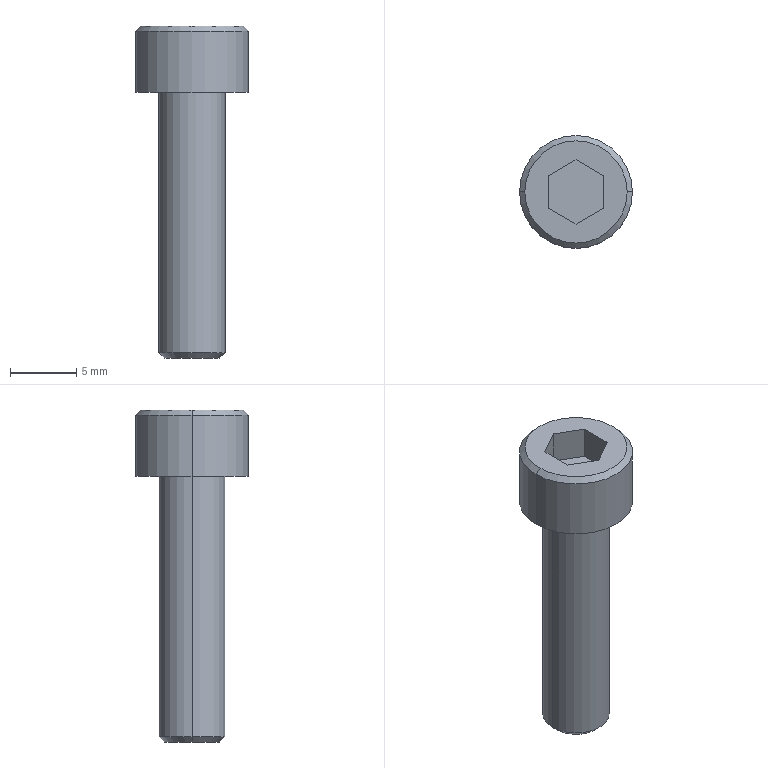Part | Creo | 1 solid | 18 faces | box 8.5 x 8.5 x 25 mm | volume 634.974 mm3 | plane 10 | cone 4 | cylinder 4 | commonest cylinder face diameters 5 x2 8.5 x2
STEP:
#1=CARTESIAN_POINT('',(95.85,150.15,32.599));
#2=VERTEX_POINT('',#1);
#3=CARTESIAN_POINT('',(88.15,150.15,32.599));
#4=VERTEX_POINT('',#3);
#5=CARTESIAN_POINT('',(92.,150.15,32.599));
#6=DIRECTION('',(0.,0.,1.));
#7=DIRECTION('',(1.,0.,0.));
#8=AXIS2_PLACEMENT_3D('',#5,#6,#7);
#9=CIRCLE('',#8,3.85);
#10=EDGE_CURVE('',#2,#4,#9,.T.);
#11=ORIENTED_EDGE('',*,*,#10,.F.);
#12=CARTESIAN_POINT('',(92.,150.15,32.599));
#13=DIRECTION('',(0.,0.,1.));
#14=DIRECTION('',(-1.,0.,0.));
#15=AXIS2_PLACEMENT_3D('',#12,#13,#14);
#16=CIRCLE('',#15,3.85);
#17=EDGE_CURVE('',#4,#2,#16,.T.);
#18=ORIENTED_EDGE('',*,*,#17,.F.);
#19=EDGE_LOOP('',(#11,#18));
#20=FACE_OUTER_BOUND('',#19,.F.);
#21=CARTESIAN_POINT('',(89.9,148.937,32.599));
#22=VERTEX_POINT('',#21);
#23=CARTESIAN_POINT('',(89.9,151.362,32.599));
#24=VERTEX_POINT('',#23);
#25=CARTESIAN_POINT('',(89.9,148.937,32.599));
#26=DIRECTION('',(0.,1.,0.));
#27=VECTOR('',#26,2.425);
#28=LINE('',#25,#27);
#29=EDGE_CURVE('',#22,#24,#28,.T.);
#30=ORIENTED_EDGE('',*,*,#29,.F.);
#31=CARTESIAN_POINT('',(92.,147.725,32.599));
#32=VERTEX_POINT('',#31);
#33=CARTESIAN_POINT('',(92.,147.725,32.599));
#34=DIRECTION('',(-0.866,0.5,0.));
#35=VECTOR('',#34,2.425);
#36=LINE('',#33,#35);
#37=EDGE_CURVE('',#32,#22,#36,.T.);
#38=ORIENTED_EDGE('',*,*,#37,.F.);
#39=CARTESIAN_POINT('',(94.1,148.937,32.599));
#40=VERTEX_POINT('',#39);
#41=CARTESIAN_POINT('',(94.1,148.937,32.599));
#42=DIRECTION('',(-0.866,-0.5,0.));
#43=VECTOR('',#42,2.425);
#44=LINE('',#41,#43);
#45=EDGE_CURVE('',#40,#32,#44,.T.);
#46=ORIENTED_EDGE('',*,*,#45,.F.);
#47=CARTESIAN_POINT('',(94.1,151.362,32.599));
#48=VERTEX_POINT('',#47);
#49=CARTESIAN_POINT('',(94.1,151.362,32.599));
#50=DIRECTION('',(0.,-1.,0.));
#51=VECTOR('',#50,2.425);
#52=LINE('',#49,#51);
#53=EDGE_CURVE('',#48,#40,#52,.T.);
#54=ORIENTED_EDGE('',*,*,#53,.F.);
#55=CARTESIAN_POINT('',(92.,152.575,32.599));
#56=VERTEX_POINT('',#55);
#57=CARTESIAN_POINT('',(92.,152.575,32.599));
#58=DIRECTION('',(0.866,-0.5,0.));
#59=VECTOR('',#58,2.425);
#60=LINE('',#57,#59);
#61=EDGE_CURVE('',#56,#48,#60,.T.);
#62=ORIENTED_EDGE('',*,*,#61,.F.);
#63=CARTESIAN_POINT('',(89.9,151.362,32.599));
#64=DIRECTION('',(0.866,0.5,0.));
#65=VECTOR('',#64,2.425);
#66=LINE('',#63,#65);
#67=EDGE_CURVE('',#24,#56,#66,.T.);
#68=ORIENTED_EDGE('',*,*,#67,.F.);
#69=EDGE_LOOP('',(#30,#38,#46,#54,#62,#68));
#70=FACE_BOUND('',#69,.F.);
#71=CARTESIAN_POINT('',(92.,150.15,32.599));
#72=DIRECTION('',(0.,0.,1.));
#73=DIRECTION('',(1.,0.,0.));
#74=AXIS2_PLACEMENT_3D('',#71,#72,#73);
#75=PLANE('',#74);
#76=ADVANCED_FACE('',(#20,#70),#75,.T.);
#77=ORIENTED_EDGE('',*,*,#10,.T.);
#78=CARTESIAN_POINT('',(87.75,150.15,32.199));
#79=VERTEX_POINT('',#78);
#80=CARTESIAN_POINT('',(88.15,150.15,32.599));
#81=DIRECTION('',(-0.7071,0.,-0.7071));
#82=VECTOR('',#81,0.5657);
#83=LINE('',#80,#82);
#84=EDGE_CURVE('',#4,#79,#83,.T.);
#85=ORIENTED_EDGE('',*,*,#84,.T.);
#86=CARTESIAN_POINT('',(96.25,150.15,32.199));
#87=VERTEX_POINT('',#86);
#88=CARTESIAN_POINT('',(92.,150.15,32.199));
#89=DIRECTION('',(0.,0.,1.));
#90=DIRECTION('',(1.,0.,0.));
#91=AXIS2_PLACEMENT_3D('',#88,#89,#90);
#92=CIRCLE('',#91,4.25);
#93=EDGE_CURVE('',#87,#79,#92,.T.);
#94=ORIENTED_EDGE('',*,*,#93,.F.);
#95=CARTESIAN_POINT('',(95.85,150.15,32.599));
#96=DIRECTION('',(0.7071,0.,-0.7071));
#97=VECTOR('',#96,0.5657);
#98=LINE('',#95,#97);
#99=EDGE_CURVE('',#2,#87,#98,.T.);
#100=ORIENTED_EDGE('',*,*,#99,.F.);
#101=EDGE_LOOP('',(#77,#85,#94,#100));
#102=FACE_OUTER_BOUND('',#101,.F.);
#103=CARTESIAN_POINT('',(92.,150.15,32.399));
#104=DIRECTION('',(0.,0.,-1.));
#105=DIRECTION('',(-1.,0.,0.));
#106=AXIS2_PLACEMENT_3D('',#103,#104,#105);
#107=CONICAL_SURFACE('',#106,4.05,45.);
#108=ADVANCED_FACE('',(#102),#107,.T.);
#109=ORIENTED_EDGE('',*,*,#17,.T.);
#110=ORIENTED_EDGE('',*,*,#99,.T.);
#111=CARTESIAN_POINT('',(92.,150.15,32.199));
#112=DIRECTION('',(0.,0.,1.));
#113=DIRECTION('',(-1.,0.,0.));
#114=AXIS2_PLACEMENT_3D('',#111,#112,#113);
#115=CIRCLE('',#114,4.25);
#116=EDGE_CURVE('',#79,#87,#115,.T.);
#117=ORIENTED_EDGE('',*,*,#116,.F.);
#118=ORIENTED_EDGE('',*,*,#84,.F.);
#119=EDGE_LOOP('',(#109,#110,#117,#118));
#120=FACE_OUTER_BOUND('',#119,.F.);
#121=CARTESIAN_POINT('',(92.,150.15,32.399));
#122=DIRECTION('',(0.,0.,-1.));
#123=DIRECTION('',(-1.,0.,0.));
#124=AXIS2_PLACEMENT_3D('',#121,#122,#123);
#125=CONICAL_SURFACE('',#124,4.05,45.);
#126=ADVANCED_FACE('',(#120),#125,.T.);
#127=ORIENTED_EDGE('',*,*,#116,.T.);
#128=CARTESIAN_POINT('',(96.25,150.15,27.599));
#129=VERTEX_POINT('',#128);
#130=CARTESIAN_POINT('',(96.25,150.15,27.599));
#131=DIRECTION('',(0.,0.,1.));
#132=VECTOR('',#131,4.6);
#133=LINE('',#130,#132);
#134=EDGE_CURVE('',#129,#87,#133,.T.);
#135=ORIENTED_EDGE('',*,*,#134,.F.);
#136=CARTESIAN_POINT('',(87.75,150.15,27.599));
#137=VERTEX_POINT('',#136);
#138=CARTESIAN_POINT('',(92.,150.15,27.599));
#139=DIRECTION('',(0.,0.,-1.));
#140=DIRECTION('',(1.,0.,0.));
#141=AXIS2_PLACEMENT_3D('',#138,#139,#140);
#142=CIRCLE('',#141,4.25);
#143=EDGE_CURVE('',#129,#137,#142,.T.);
#144=ORIENTED_EDGE('',*,*,#143,.T.);
#145=CARTESIAN_POINT('',(87.75,150.15,27.599));
#146=DIRECTION('',(0.,0.,1.));
#147=VECTOR('',#146,4.6);
#148=LINE('',#145,#147);
#149=EDGE_CURVE('',#137,#79,#148,.T.);
#150=ORIENTED_EDGE('',*,*,#149,.T.);
#151=EDGE_LOOP('',(#127,#135,#144,#150));
#152=FACE_OUTER_BOUND('',#151,.F.);
#153=CARTESIAN_POINT('',(92.,150.15,27.599));
#154=DIRECTION('',(0.,0.,1.));
#155=DIRECTION('',(1.,0.,0.));
#156=AXIS2_PLACEMENT_3D('',#153,#154,#155);
#157=CYLINDRICAL_SURFACE('',#156,4.25);
#158=ADVANCED_FACE('',(#152),#157,.T.);
#159=ORIENTED_EDGE('',*,*,#93,.T.);
#160=ORIENTED_EDGE('',*,*,#149,.F.);
#161=CARTESIAN_POINT('',(92.,150.15,27.599));
#162=DIRECTION('',(0.,0.,-1.));
#163=DIRECTION('',(-1.,0.,0.));
#164=AXIS2_PLACEMENT_3D('',#161,#162,#163);
#165=CIRCLE('',#164,4.25);
#166=EDGE_CURVE('',#137,#129,#165,.T.);
#167=ORIENTED_EDGE('',*,*,#166,.T.);
#168=ORIENTED_EDGE('',*,*,#134,.T.);
#169=EDGE_LOOP('',(#159,#160,#167,#168));
#170=FACE_OUTER_BOUND('',#169,.F.);
#171=CARTESIAN_POINT('',(92.,150.15,27.599));
#172=DIRECTION('',(0.,0.,1.));
#173=DIRECTION('',(1.,0.,0.));
#174=AXIS2_PLACEMENT_3D('',#171,#172,#173);
#175=CYLINDRICAL_SURFACE('',#174,4.25);
#176=ADVANCED_FACE('',(#170),#175,.T.);
#177=ORIENTED_EDGE('',*,*,#143,.F.);
#178=ORIENTED_EDGE('',*,*,#166,.F.);
#179=EDGE_LOOP('',(#177,#178));
#180=FACE_OUTER_BOUND('',#179,.F.);
#181=CARTESIAN_POINT('',(89.5,150.15,27.599));
#182=VERTEX_POINT('',#181);
#183=CARTESIAN_POINT('',(94.5,150.15,27.599));
#184=VERTEX_POINT('',#183);
#185=CARTESIAN_POINT('',(92.,150.15,27.599));
#186=DIRECTION('',(0.,0.,1.));
#187=DIRECTION('',(-1.,0.,0.));
#188=AXIS2_PLACEMENT_3D('',#185,#186,#187);
#189=CIRCLE('',#188,2.5);
#190=EDGE_CURVE('',#182,#184,#189,.T.);
#191=ORIENTED_EDGE('',*,*,#190,.F.);
#192=CARTESIAN_POINT('',(92.,150.15,27.599));
#193=DIRECTION('',(0.,0.,1.));
#194=DIRECTION('',(1.,0.,0.));
#195=AXIS2_PLACEMENT_3D('',#192,#193,#194);
#196=CIRCLE('',#195,2.5);
#197=EDGE_CURVE('',#184,#182,#196,.T.);
#198=ORIENTED_EDGE('',*,*,#197,.F.);
#199=EDGE_LOOP('',(#191,#198));
#200=FACE_BOUND('',#199,.F.);
#201=CARTESIAN_POINT('',(92.,150.15,27.599));
#202=DIRECTION('',(0.,0.,-1.));
#203=DIRECTION('',(-1.,0.,0.));
#204=AXIS2_PLACEMENT_3D('',#201,#202,#203);
#205=PLANE('',#204);
#206=ADVANCED_FACE('',(#180,#200),#205,.T.);
#207=CARTESIAN_POINT('',(94.5,150.15,7.999));
#208=VERTEX_POINT('',#207);
#209=CARTESIAN_POINT('',(89.5,150.15,7.999));
#210=VERTEX_POINT('',#209);
#211=CARTESIAN_POINT('',(92.,150.15,7.999));
#212=DIRECTION('',(0.,0.,-1.));
#213=DIRECTION('',(1.,0.,0.));
#214=AXIS2_PLACEMENT_3D('',#211,#212,#213);
#215=CIRCLE('',#214,2.5);
#216=EDGE_CURVE('',#208,#210,#215,.T.);
#217=ORIENTED_EDGE('',*,*,#216,.T.);
#218=CARTESIAN_POINT('',(89.5,150.15,27.599));
#219=DIRECTION('',(0.,0.,-1.));
#220=VECTOR('',#219,19.6);
#221=LINE('',#218,#220);
#222=EDGE_CURVE('',#182,#210,#221,.T.);
#223=ORIENTED_EDGE('',*,*,#222,.F.);
#224=ORIENTED_EDGE('',*,*,#190,.T.);
#225=CARTESIAN_POINT('',(94.5,150.15,27.599));
#226=DIRECTION('',(0.,0.,-1.));
#227=VECTOR('',#226,19.6);
#228=LINE('',#225,#227);
#229=EDGE_CURVE('',#184,#208,#228,.T.);
#230=ORIENTED_EDGE('',*,*,#229,.T.);
#231=EDGE_LOOP('',(#217,#223,#224,#230));
#232=FACE_OUTER_BOUND('',#231,.F.);
#233=CARTESIAN_POINT('',(92.,150.15,27.599));
#234=DIRECTION('',(0.,0.,-1.));
#235=DIRECTION('',(-1.,0.,0.));
#236=AXIS2_PLACEMENT_3D('',#233,#234,#235);
#237=CYLINDRICAL_SURFACE('',#236,2.5);
#238=ADVANCED_FACE('',(#232),#237,.T.);
#239=CARTESIAN_POINT('',(94.1,150.15,7.599));
#240=VERTEX_POINT('',#239);
#241=CARTESIAN_POINT('',(89.9,150.15,7.599));
#242=VERTEX_POINT('',#241);
#243=CARTESIAN_POINT('',(92.,150.15,7.599));
#244=DIRECTION('',(0.,0.,-1.));
#245=DIRECTION('',(1.,0.,0.));
#246=AXIS2_PLACEMENT_3D('',#243,#244,#245);
#247=CIRCLE('',#246,2.1);
#248=EDGE_CURVE('',#240,#242,#247,.T.);
#249=ORIENTED_EDGE('',*,*,#248,.T.);
#250=CARTESIAN_POINT('',(89.9,150.15,7.599));
#251=DIRECTION('',(-0.7071,0.,0.7071));
#252=VECTOR('',#251,0.5657);
#253=LINE('',#250,#252);
#254=EDGE_CURVE('',#242,#210,#253,.T.);
#255=ORIENTED_EDGE('',*,*,#254,.T.);
#256=ORIENTED_EDGE('',*,*,#216,.F.);
#257=CARTESIAN_POINT('',(94.1,150.15,7.599));
#258=DIRECTION('',(0.7071,0.,0.7071));
#259=VECTOR('',#258,0.5657);
#260=LINE('',#257,#259);
#261=EDGE_CURVE('',#240,#208,#260,.T.);
#262=ORIENTED_EDGE('',*,*,#261,.F.);
#263=EDGE_LOOP('',(#249,#255,#256,#262));
#264=FACE_OUTER_BOUND('',#263,.F.);
#265=CARTESIAN_POINT('',(92.,150.15,7.799));
#266=DIRECTION('',(0.,0.,1.));
#267=DIRECTION('',(1.,0.,0.));
#268=AXIS2_PLACEMENT_3D('',#265,#266,#267);
#269=CONICAL_SURFACE('',#268,2.3,45.);
#270=ADVANCED_FACE('',(#264),#269,.T.);
#271=CARTESIAN_POINT('',(92.,150.15,7.599));
#272=DIRECTION('',(0.,0.,-1.));
#273=DIRECTION('',(-1.,0.,0.));
#274=AXIS2_PLACEMENT_3D('',#271,#272,#273);
#275=CIRCLE('',#274,2.1);
#276=EDGE_CURVE('',#242,#240,#275,.T.);
#277=ORIENTED_EDGE('',*,*,#276,.F.);
#278=ORIENTED_EDGE('',*,*,#248,.F.);
#279=EDGE_LOOP('',(#277,#278));
#280=FACE_OUTER_BOUND('',#279,.F.);
#281=CARTESIAN_POINT('',(92.,150.15,7.599));
#282=DIRECTION('',(0.,0.,-1.));
#283=DIRECTION('',(-1.,0.,0.));
#284=AXIS2_PLACEMENT_3D('',#281,#282,#283);
#285=PLANE('',#284);
#286=ADVANCED_FACE('',(#280),#285,.T.);
#287=ORIENTED_EDGE('',*,*,#276,.T.);
#288=ORIENTED_EDGE('',*,*,#261,.T.);
#289=CARTESIAN_POINT('',(92.,150.15,7.999));
#290=DIRECTION('',(0.,0.,-1.));
#291=DIRECTION('',(-1.,0.,0.));
#292=AXIS2_PLACEMENT_3D('',#289,#290,#291);
#293=CIRCLE('',#292,2.5);
#294=EDGE_CURVE('',#210,#208,#293,.T.);
#295=ORIENTED_EDGE('',*,*,#294,.F.);
#296=ORIENTED_EDGE('',*,*,#254,.F.);
#297=EDGE_LOOP('',(#287,#288,#295,#296));
#298=FACE_OUTER_BOUND('',#297,.F.);
#299=CARTESIAN_POINT('',(92.,150.15,7.799));
#300=DIRECTION('',(0.,0.,1.));
#301=DIRECTION('',(1.,0.,0.));
#302=AXIS2_PLACEMENT_3D('',#299,#300,#301);
#303=CONICAL_SURFACE('',#302,2.3,45.);
#304=ADVANCED_FACE('',(#298),#303,.T.);
#305=ORIENTED_EDGE('',*,*,#294,.T.);
#306=ORIENTED_EDGE('',*,*,#229,.F.);
#307=ORIENTED_EDGE('',*,*,#197,.T.);
#308=ORIENTED_EDGE('',*,*,#222,.T.);
#309=EDGE_LOOP('',(#305,#306,#307,#308));
#310=FACE_OUTER_BOUND('',#309,.F.);
#311=CARTESIAN_POINT('',(92.,150.15,27.599));
#312=DIRECTION('',(0.,0.,-1.));
#313=DIRECTION('',(-1.,0.,0.));
#314=AXIS2_PLACEMENT_3D('',#311,#312,#313);
#315=CYLINDRICAL_SURFACE('',#314,2.5);
#316=ADVANCED_FACE('',(#310),#315,.T.);
#317=ORIENTED_EDGE('',*,*,#29,.T.);
#318=CARTESIAN_POINT('',(89.9,151.362,30.099));
#319=VERTEX_POINT('',#318);
#320=CARTESIAN_POINT('',(89.9,151.362,32.599));
#321=DIRECTION('',(0.,0.,-1.));
#322=VECTOR('',#321,2.5);
#323=LINE('',#320,#322);
#324=EDGE_CURVE('',#24,#319,#323,.T.);
#325=ORIENTED_EDGE('',*,*,#324,.T.);
#326=CARTESIAN_POINT('',(89.9,148.937,30.099));
#327=VERTEX_POINT('',#326);
#328=CARTESIAN_POINT('',(89.9,148.937,30.099));
#329=DIRECTION('',(0.,1.,0.));
#330=VECTOR('',#329,2.425);
#331=LINE('',#328,#330);
#332=EDGE_CURVE('',#327,#319,#331,.T.);
#333=ORIENTED_EDGE('',*,*,#332,.F.);
#334=CARTESIAN_POINT('',(89.9,148.937,32.599));
#335=DIRECTION('',(0.,0.,-1.));
#336=VECTOR('',#335,2.5);
#337=LINE('',#334,#336);
#338=EDGE_CURVE('',#22,#327,#337,.T.);
#339=ORIENTED_EDGE('',*,*,#338,.F.);
#340=EDGE_LOOP('',(#317,#325,#333,#339));
#341=FACE_OUTER_BOUND('',#340,.F.);
#342=CARTESIAN_POINT('',(89.9,150.15,31.349));
#343=DIRECTION('',(-1.,0.,0.));
#344=DIRECTION('',(0.,0.,1.));
#345=AXIS2_PLACEMENT_3D('',#342,#343,#344);
#346=PLANE('',#345);
#347=ADVANCED_FACE('',(#341),#346,.F.);
#348=ORIENTED_EDGE('',*,*,#67,.T.);
#349=CARTESIAN_POINT('',(92.,152.575,30.099));
#350=VERTEX_POINT('',#349);
#351=CARTESIAN_POINT('',(92.,152.575,32.599));
#352=DIRECTION('',(0.,0.,-1.));
#353=VECTOR('',#352,2.5);
#354=LINE('',#351,#353);
#355=EDGE_CURVE('',#56,#350,#354,.T.);
#356=ORIENTED_EDGE('',*,*,#355,.T.);
#357=CARTESIAN_POINT('',(92.,152.575,30.099));
#358=DIRECTION('',(-0.866,-0.5,0.));
#359=VECTOR('',#358,2.425);
#360=LINE('',#357,#359);
#361=EDGE_CURVE('',#350,#319,#360,.T.);
#362=ORIENTED_EDGE('',*,*,#361,.T.);
#363=ORIENTED_EDGE('',*,*,#324,.F.);
#364=EDGE_LOOP('',(#348,#356,#362,#363));
#365=FACE_OUTER_BOUND('',#364,.F.);
#366=CARTESIAN_POINT('',(90.95,151.968,31.349));
#367=DIRECTION('',(-0.5,0.866,0.));
#368=DIRECTION('',(-0.866,-0.5,0.));
#369=AXIS2_PLACEMENT_3D('',#366,#367,#368);
#370=PLANE('',#369);
#371=ADVANCED_FACE('',(#365),#370,.F.);
#372=ORIENTED_EDGE('',*,*,#61,.T.);
#373=CARTESIAN_POINT('',(94.1,151.362,30.099));
#374=VERTEX_POINT('',#373);
#375=CARTESIAN_POINT('',(94.1,151.362,32.599));
#376=DIRECTION('',(0.,0.,-1.));
#377=VECTOR('',#376,2.5);
#378=LINE('',#375,#377);
#379=EDGE_CURVE('',#48,#374,#378,.T.);
#380=ORIENTED_EDGE('',*,*,#379,.T.);
#381=CARTESIAN_POINT('',(94.1,151.362,30.099));
#382=DIRECTION('',(-0.866,0.5,0.));
#383=VECTOR('',#382,2.425);
#384=LINE('',#381,#383);
#385=EDGE_CURVE('',#374,#350,#384,.T.);
#386=ORIENTED_EDGE('',*,*,#385,.T.);
#387=ORIENTED_EDGE('',*,*,#355,.F.);
#388=EDGE_LOOP('',(#372,#380,#386,#387));
#389=FACE_OUTER_BOUND('',#388,.F.);
#390=CARTESIAN_POINT('',(93.05,151.968,31.349));
#391=DIRECTION('',(0.5,0.866,0.));
#392=DIRECTION('',(-0.866,0.5,0.));
#393=AXIS2_PLACEMENT_3D('',#390,#391,#392);
#394=PLANE('',#393);
#395=ADVANCED_FACE('',(#389),#394,.F.);
#396=ORIENTED_EDGE('',*,*,#53,.T.);
#397=CARTESIAN_POINT('',(94.1,148.937,30.099));
#398=VERTEX_POINT('',#397);
#399=CARTESIAN_POINT('',(94.1,148.937,32.599));
#400=DIRECTION('',(0.,0.,-1.));
#401=VECTOR('',#400,2.5);
#402=LINE('',#399,#401);
#403=EDGE_CURVE('',#40,#398,#402,.T.);
#404=ORIENTED_EDGE('',*,*,#403,.T.);
#405=CARTESIAN_POINT('',(94.1,151.362,30.099));
#406=DIRECTION('',(0.,-1.,0.));
#407=VECTOR('',#406,2.425);
#408=LINE('',#405,#407);
#409=EDGE_CURVE('',#374,#398,#408,.T.);
#410=ORIENTED_EDGE('',*,*,#409,.F.);
#411=ORIENTED_EDGE('',*,*,#379,.F.);
#412=EDGE_LOOP('',(#396,#404,#410,#411));
#413=FACE_OUTER_BOUND('',#412,.F.);
#414=CARTESIAN_POINT('',(94.1,150.15,31.349));
#415=DIRECTION('',(1.,0.,0.));
#416=DIRECTION('',(0.,0.,-1.));
#417=AXIS2_PLACEMENT_3D('',#414,#415,#416);
#418=PLANE('',#417);
#419=ADVANCED_FACE('',(#413),#418,.F.);
#420=ORIENTED_EDGE('',*,*,#45,.T.);
#421=CARTESIAN_POINT('',(92.,147.725,30.099));
#422=VERTEX_POINT('',#421);
#423=CARTESIAN_POINT('',(92.,147.725,32.599));
#424=DIRECTION('',(0.,0.,-1.));
#425=VECTOR('',#424,2.5);
#426=LINE('',#423,#425);
#427=EDGE_CURVE('',#32,#422,#426,.T.);
#428=ORIENTED_EDGE('',*,*,#427,.T.);
#429=CARTESIAN_POINT('',(92.,147.725,30.099));
#430=DIRECTION('',(0.866,0.5,0.));
#431=VECTOR('',#430,2.425);
#432=LINE('',#429,#431);
#433=EDGE_CURVE('',#422,#398,#432,.T.);
#434=ORIENTED_EDGE('',*,*,#433,.T.);
#435=ORIENTED_EDGE('',*,*,#403,.F.);
#436=EDGE_LOOP('',(#420,#428,#434,#435));
#437=FACE_OUTER_BOUND('',#436,.F.);
#438=CARTESIAN_POINT('',(93.05,148.331,31.349));
#439=DIRECTION('',(0.5,-0.866,0.));
#440=DIRECTION('',(0.866,0.5,0.));
#441=AXIS2_PLACEMENT_3D('',#438,#439,#440);
#442=PLANE('',#441);
#443=ADVANCED_FACE('',(#437),#442,.F.);
#444=ORIENTED_EDGE('',*,*,#37,.T.);
#445=ORIENTED_EDGE('',*,*,#338,.T.);
#446=CARTESIAN_POINT('',(89.9,148.937,30.099));
#447=DIRECTION('',(0.866,-0.5,0.));
#448=VECTOR('',#447,2.425);
#449=LINE('',#446,#448);
#450=EDGE_CURVE('',#327,#422,#449,.T.);
#451=ORIENTED_EDGE('',*,*,#450,.T.);
#452=ORIENTED_EDGE('',*,*,#427,.F.);
#453=EDGE_LOOP('',(#444,#445,#451,#452));
#454=FACE_OUTER_BOUND('',#453,.F.);
#455=CARTESIAN_POINT('',(90.95,148.331,31.349));
#456=DIRECTION('',(-0.5,-0.866,0.));
#457=DIRECTION('',(0.866,-0.5,0.));
#458=AXIS2_PLACEMENT_3D('',#455,#456,#457);
#459=PLANE('',#458);
#460=ADVANCED_FACE('',(#454),#459,.F.);
#461=ORIENTED_EDGE('',*,*,#433,.F.);
#462=ORIENTED_EDGE('',*,*,#450,.F.);
#463=ORIENTED_EDGE('',*,*,#332,.T.);
#464=ORIENTED_EDGE('',*,*,#361,.F.);
#465=ORIENTED_EDGE('',*,*,#385,.F.);
#466=ORIENTED_EDGE('',*,*,#409,.T.);
#467=EDGE_LOOP('',(#461,#462,#463,#464,#465,#466));
#468=FACE_OUTER_BOUND('',#467,.F.);
#469=CARTESIAN_POINT('',(92.,150.15,30.099));
#470=DIRECTION('',(0.,0.,-1.));
#471=DIRECTION('',(-1.,0.,0.));
#472=AXIS2_PLACEMENT_3D('',#469,#470,#471);
#473=PLANE('',#472);
#474=ADVANCED_FACE('',(#468),#473,.F.);
#475=CLOSED_SHELL('',(#76,#108,#126,#158,#176,#206,#238,#270,#286,#304,#316,#347,#371,#395,#419,#443,#460,#474));
#476=MANIFOLD_SOLID_BREP('',#475);
#477=(LENGTH_UNIT()NAMED_UNIT(*)SI_UNIT(.MILLI.,.METRE.));
#478=UNCERTAINTY_MEASURE_WITH_UNIT(LENGTH_MEASURE(0.002774),#477,'','');
#479=(NAMED_UNIT(*)PLANE_ANGLE_UNIT()SI_UNIT($,.RADIAN.));
#480=PLANE_ANGLE_MEASURE_WITH_UNIT(PLANE_ANGLE_MEASURE(0.01745),#479);
#481=(CONVERSION_BASED_UNIT('DEGREE',#480)NAMED_UNIT(*)PLANE_ANGLE_UNIT());
#482=(NAMED_UNIT(*)SI_UNIT($,.STERADIAN.)SOLID_ANGLE_UNIT());
#483=(GEOMETRIC_REPRESENTATION_CONTEXT(3)GLOBAL_UNCERTAINTY_ASSIGNED_CONTEXT((#478))GLOBAL_UNIT_ASSIGNED_CONTEXT((#477,#481,#482))REPRESENTATION_CONTEXT('',''));
#484=ADVANCED_BREP_SHAPE_REPRESENTATION('',(#476),#483);